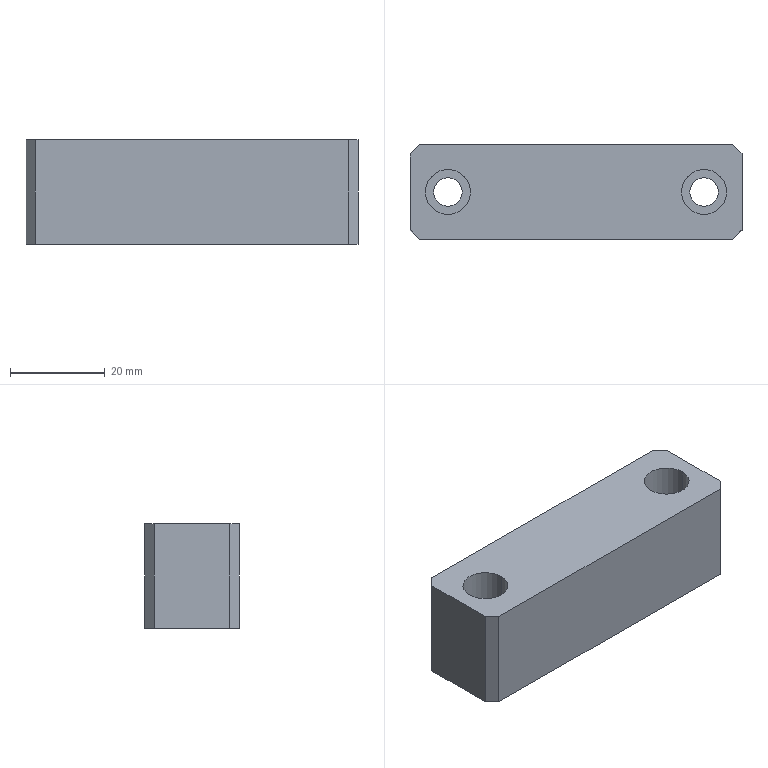Part | SolidWorks | features Chamfer 1, Extrusion 1, HoleWzd 1 | 1 solid | 20 faces | box 70 x 20 x 22 mm | volume 28656 mm3 | plane 12 | cylinder 8 | commonest cylinder face diameters 6 x4 9.5 x4
STEP:
#1=CARTESIAN_POINT('',(-29.44,2.003,1.5));
#2=VERTEX_POINT('',#1);
#3=CARTESIAN_POINT('',(-19.94,2.003,1.5));
#4=VERTEX_POINT('',#3);
#5=CARTESIAN_POINT('',(-24.69,2.003,1.5));
#6=DIRECTION('',(0.,0.,1.));
#7=DIRECTION('',(1.,0.,0.));
#8=AXIS2_PLACEMENT_3D('',#5,#6,#7);
#9=CIRCLE('',#8,4.75);
#10=EDGE_CURVE('',#2,#4,#9,.T.);
#11=ORIENTED_EDGE('',*,*,#10,.F.);
#12=CARTESIAN_POINT('',(-29.44,2.003,10.));
#13=VERTEX_POINT('',#12);
#14=CARTESIAN_POINT('',(-29.44,2.003,10.));
#15=DIRECTION('',(0.,0.,1.));
#16=VECTOR('',#15,1000.);
#17=LINE('',#14,#16);
#18=EDGE_CURVE('',#2,#13,#17,.T.);
#19=ORIENTED_EDGE('',*,*,#18,.T.);
#20=CARTESIAN_POINT('',(-19.94,2.003,10.));
#21=VERTEX_POINT('',#20);
#22=CARTESIAN_POINT('',(-24.69,2.003,10.));
#23=DIRECTION('',(0.,0.,1.));
#24=DIRECTION('',(1.,0.,0.));
#25=AXIS2_PLACEMENT_3D('',#22,#23,#24);
#26=CIRCLE('',#25,4.75);
#27=EDGE_CURVE('',#13,#21,#26,.T.);
#28=ORIENTED_EDGE('',*,*,#27,.T.);
#29=CARTESIAN_POINT('',(-19.94,2.003,10.));
#30=DIRECTION('',(0.,0.,1.));
#31=VECTOR('',#30,1000.);
#32=LINE('',#29,#31);
#33=EDGE_CURVE('',#4,#21,#32,.T.);
#34=ORIENTED_EDGE('',*,*,#33,.F.);
#35=EDGE_LOOP('',(#11,#19,#28,#34));
#36=FACE_OUTER_BOUND('',#35,.T.);
#37=CARTESIAN_POINT('',(-24.69,2.003,10.));
#38=DIRECTION('',(0.,0.,1.));
#39=DIRECTION('',(1.,0.,0.));
#40=AXIS2_PLACEMENT_3D('',#37,#38,#39);
#41=CYLINDRICAL_SURFACE('',#40,4.75);
#42=ADVANCED_FACE('',(#36),#41,.F.);
#43=CARTESIAN_POINT('',(-27.69,2.003,-12.));
#44=VERTEX_POINT('',#43);
#45=CARTESIAN_POINT('',(-21.69,2.003,-12.));
#46=VERTEX_POINT('',#45);
#47=CARTESIAN_POINT('',(-24.69,2.003,-12.));
#48=DIRECTION('',(0.,0.,1.));
#49=DIRECTION('',(1.,0.,0.));
#50=AXIS2_PLACEMENT_3D('',#47,#48,#49);
#51=CIRCLE('',#50,3.);
#52=EDGE_CURVE('',#44,#46,#51,.T.);
#53=ORIENTED_EDGE('',*,*,#52,.F.);
#54=CARTESIAN_POINT('',(-27.69,2.003,1.5));
#55=VERTEX_POINT('',#54);
#56=CARTESIAN_POINT('',(-27.69,2.003,10.));
#57=DIRECTION('',(0.,0.,1.));
#58=VECTOR('',#57,1000.);
#59=LINE('',#56,#58);
#60=EDGE_CURVE('',#44,#55,#59,.T.);
#61=ORIENTED_EDGE('',*,*,#60,.T.);
#62=CARTESIAN_POINT('',(-21.69,2.003,1.5));
#63=VERTEX_POINT('',#62);
#64=CARTESIAN_POINT('',(-24.69,2.003,1.5));
#65=DIRECTION('',(0.,0.,1.));
#66=DIRECTION('',(1.,0.,0.));
#67=AXIS2_PLACEMENT_3D('',#64,#65,#66);
#68=CIRCLE('',#67,3.);
#69=EDGE_CURVE('',#55,#63,#68,.T.);
#70=ORIENTED_EDGE('',*,*,#69,.T.);
#71=CARTESIAN_POINT('',(-21.69,2.003,10.));
#72=DIRECTION('',(0.,0.,1.));
#73=VECTOR('',#72,1000.);
#74=LINE('',#71,#73);
#75=EDGE_CURVE('',#46,#63,#74,.T.);
#76=ORIENTED_EDGE('',*,*,#75,.F.);
#77=EDGE_LOOP('',(#53,#61,#70,#76));
#78=FACE_OUTER_BOUND('',#77,.T.);
#79=CARTESIAN_POINT('',(-24.69,2.003,10.));
#80=DIRECTION('',(0.,0.,1.));
#81=DIRECTION('',(1.,0.,0.));
#82=AXIS2_PLACEMENT_3D('',#79,#80,#81);
#83=CYLINDRICAL_SURFACE('',#82,3.);
#84=ADVANCED_FACE('',(#78),#83,.F.);
#85=CARTESIAN_POINT('',(24.56,2.003,1.5));
#86=VERTEX_POINT('',#85);
#87=CARTESIAN_POINT('',(34.06,2.003,1.5));
#88=VERTEX_POINT('',#87);
#89=CARTESIAN_POINT('',(29.31,2.003,1.5));
#90=DIRECTION('',(0.,0.,1.));
#91=DIRECTION('',(1.,0.,0.));
#92=AXIS2_PLACEMENT_3D('',#89,#90,#91);
#93=CIRCLE('',#92,4.75);
#94=EDGE_CURVE('',#86,#88,#93,.T.);
#95=ORIENTED_EDGE('',*,*,#94,.F.);
#96=CARTESIAN_POINT('',(24.56,2.003,10.));
#97=VERTEX_POINT('',#96);
#98=CARTESIAN_POINT('',(24.56,2.003,10.));
#99=DIRECTION('',(0.,0.,1.));
#100=VECTOR('',#99,1000.);
#101=LINE('',#98,#100);
#102=EDGE_CURVE('',#86,#97,#101,.T.);
#103=ORIENTED_EDGE('',*,*,#102,.T.);
#104=CARTESIAN_POINT('',(34.06,2.003,10.));
#105=VERTEX_POINT('',#104);
#106=CARTESIAN_POINT('',(29.31,2.003,10.));
#107=DIRECTION('',(0.,0.,1.));
#108=DIRECTION('',(1.,0.,0.));
#109=AXIS2_PLACEMENT_3D('',#106,#107,#108);
#110=CIRCLE('',#109,4.75);
#111=EDGE_CURVE('',#97,#105,#110,.T.);
#112=ORIENTED_EDGE('',*,*,#111,.T.);
#113=CARTESIAN_POINT('',(34.06,2.003,10.));
#114=DIRECTION('',(0.,0.,1.));
#115=VECTOR('',#114,1000.);
#116=LINE('',#113,#115);
#117=EDGE_CURVE('',#88,#105,#116,.T.);
#118=ORIENTED_EDGE('',*,*,#117,.F.);
#119=EDGE_LOOP('',(#95,#103,#112,#118));
#120=FACE_OUTER_BOUND('',#119,.T.);
#121=CARTESIAN_POINT('',(29.31,2.003,10.));
#122=DIRECTION('',(0.,0.,1.));
#123=DIRECTION('',(1.,0.,0.));
#124=AXIS2_PLACEMENT_3D('',#121,#122,#123);
#125=CYLINDRICAL_SURFACE('',#124,4.75);
#126=ADVANCED_FACE('',(#120),#125,.F.);
#127=CARTESIAN_POINT('',(26.31,2.003,-12.));
#128=VERTEX_POINT('',#127);
#129=CARTESIAN_POINT('',(32.31,2.003,-12.));
#130=VERTEX_POINT('',#129);
#131=CARTESIAN_POINT('',(29.31,2.003,-12.));
#132=DIRECTION('',(0.,0.,1.));
#133=DIRECTION('',(1.,0.,0.));
#134=AXIS2_PLACEMENT_3D('',#131,#132,#133);
#135=CIRCLE('',#134,3.);
#136=EDGE_CURVE('',#128,#130,#135,.T.);
#137=ORIENTED_EDGE('',*,*,#136,.F.);
#138=CARTESIAN_POINT('',(26.31,2.003,1.5));
#139=VERTEX_POINT('',#138);
#140=CARTESIAN_POINT('',(26.31,2.003,10.));
#141=DIRECTION('',(0.,0.,1.));
#142=VECTOR('',#141,1000.);
#143=LINE('',#140,#142);
#144=EDGE_CURVE('',#128,#139,#143,.T.);
#145=ORIENTED_EDGE('',*,*,#144,.T.);
#146=CARTESIAN_POINT('',(32.31,2.003,1.5));
#147=VERTEX_POINT('',#146);
#148=CARTESIAN_POINT('',(29.31,2.003,1.5));
#149=DIRECTION('',(0.,0.,1.));
#150=DIRECTION('',(1.,0.,0.));
#151=AXIS2_PLACEMENT_3D('',#148,#149,#150);
#152=CIRCLE('',#151,3.);
#153=EDGE_CURVE('',#139,#147,#152,.T.);
#154=ORIENTED_EDGE('',*,*,#153,.T.);
#155=CARTESIAN_POINT('',(32.31,2.003,10.));
#156=DIRECTION('',(0.,0.,1.));
#157=VECTOR('',#156,1000.);
#158=LINE('',#155,#157);
#159=EDGE_CURVE('',#130,#147,#158,.T.);
#160=ORIENTED_EDGE('',*,*,#159,.F.);
#161=EDGE_LOOP('',(#137,#145,#154,#160));
#162=FACE_OUTER_BOUND('',#161,.T.);
#163=CARTESIAN_POINT('',(29.31,2.003,10.));
#164=DIRECTION('',(0.,0.,1.));
#165=DIRECTION('',(1.,0.,0.));
#166=AXIS2_PLACEMENT_3D('',#163,#164,#165);
#167=CYLINDRICAL_SURFACE('',#166,3.);
#168=ADVANCED_FACE('',(#162),#167,.F.);
#169=CARTESIAN_POINT('',(-32.69,10.003,-12.));
#170=VERTEX_POINT('',#169);
#171=CARTESIAN_POINT('',(-32.69,-5.997,-12.));
#172=VERTEX_POINT('',#171);
#173=CARTESIAN_POINT('',(-32.69,12.003,-12.));
#174=DIRECTION('',(0.,-1.,0.));
#175=VECTOR('',#174,1000.);
#176=LINE('',#173,#175);
#177=EDGE_CURVE('',#170,#172,#176,.T.);
#178=ORIENTED_EDGE('',*,*,#177,.T.);
#179=CARTESIAN_POINT('',(-32.69,-5.997,10.));
#180=VERTEX_POINT('',#179);
#181=CARTESIAN_POINT('',(-32.69,-5.997,-12.));
#182=DIRECTION('',(0.,0.,1.));
#183=VECTOR('',#182,1000.);
#184=LINE('',#181,#183);
#185=EDGE_CURVE('',#172,#180,#184,.T.);
#186=ORIENTED_EDGE('',*,*,#185,.T.);
#187=CARTESIAN_POINT('',(-32.69,10.003,10.));
#188=VERTEX_POINT('',#187);
#189=CARTESIAN_POINT('',(-32.69,12.003,10.));
#190=DIRECTION('',(0.,-1.,0.));
#191=VECTOR('',#190,1000.);
#192=LINE('',#189,#191);
#193=EDGE_CURVE('',#188,#180,#192,.T.);
#194=ORIENTED_EDGE('',*,*,#193,.F.);
#195=CARTESIAN_POINT('',(-32.69,10.003,-12.));
#196=DIRECTION('',(0.,0.,-1.));
#197=VECTOR('',#196,1000.);
#198=LINE('',#195,#197);
#199=EDGE_CURVE('',#188,#170,#198,.T.);
#200=ORIENTED_EDGE('',*,*,#199,.T.);
#201=EDGE_LOOP('',(#178,#186,#194,#200));
#202=FACE_OUTER_BOUND('',#201,.T.);
#203=CARTESIAN_POINT('',(-32.69,12.003,-12.));
#204=DIRECTION('',(-1.,0.,0.));
#205=DIRECTION('',(0.,-1.,0.));
#206=AXIS2_PLACEMENT_3D('',#203,#204,#205);
#207=PLANE('',#206);
#208=ADVANCED_FACE('',(#202),#207,.T.);
#209=CARTESIAN_POINT('',(35.31,12.003,10.));
#210=VERTEX_POINT('',#209);
#211=CARTESIAN_POINT('',(-30.69,12.003,10.));
#212=VERTEX_POINT('',#211);
#213=CARTESIAN_POINT('',(-32.69,12.003,10.));
#214=DIRECTION('',(-1.,0.,0.));
#215=VECTOR('',#214,1000.);
#216=LINE('',#213,#215);
#217=EDGE_CURVE('',#210,#212,#216,.T.);
#218=ORIENTED_EDGE('',*,*,#217,.F.);
#219=CARTESIAN_POINT('',(35.31,12.003,-12.));
#220=VERTEX_POINT('',#219);
#221=CARTESIAN_POINT('',(35.31,12.003,-12.));
#222=DIRECTION('',(0.,0.,-1.));
#223=VECTOR('',#222,1000.);
#224=LINE('',#221,#223);
#225=EDGE_CURVE('',#210,#220,#224,.T.);
#226=ORIENTED_EDGE('',*,*,#225,.T.);
#227=CARTESIAN_POINT('',(-30.69,12.003,-12.));
#228=VERTEX_POINT('',#227);
#229=CARTESIAN_POINT('',(-32.69,12.003,-12.));
#230=DIRECTION('',(-1.,0.,0.));
#231=VECTOR('',#230,1000.);
#232=LINE('',#229,#231);
#233=EDGE_CURVE('',#220,#228,#232,.T.);
#234=ORIENTED_EDGE('',*,*,#233,.T.);
#235=CARTESIAN_POINT('',(-30.69,12.003,-12.));
#236=DIRECTION('',(0.,0.,1.));
#237=VECTOR('',#236,1000.);
#238=LINE('',#235,#237);
#239=EDGE_CURVE('',#228,#212,#238,.T.);
#240=ORIENTED_EDGE('',*,*,#239,.T.);
#241=EDGE_LOOP('',(#218,#226,#234,#240));
#242=FACE_OUTER_BOUND('',#241,.T.);
#243=CARTESIAN_POINT('',(-32.69,12.003,-12.));
#244=DIRECTION('',(0.,1.,0.));
#245=DIRECTION('',(0.,0.,1.));
#246=AXIS2_PLACEMENT_3D('',#243,#244,#245);
#247=PLANE('',#246);
#248=ADVANCED_FACE('',(#242),#247,.T.);
#249=CARTESIAN_POINT('',(37.31,-5.997,10.));
#250=VERTEX_POINT('',#249);
#251=CARTESIAN_POINT('',(37.31,10.003,10.));
#252=VERTEX_POINT('',#251);
#253=CARTESIAN_POINT('',(37.31,12.003,10.));
#254=DIRECTION('',(0.,1.,0.));
#255=VECTOR('',#254,1000.);
#256=LINE('',#253,#255);
#257=EDGE_CURVE('',#250,#252,#256,.T.);
#258=ORIENTED_EDGE('',*,*,#257,.F.);
#259=CARTESIAN_POINT('',(37.31,-5.997,-12.));
#260=VERTEX_POINT('',#259);
#261=CARTESIAN_POINT('',(37.31,-5.997,-12.));
#262=DIRECTION('',(0.,0.,-1.));
#263=VECTOR('',#262,1000.);
#264=LINE('',#261,#263);
#265=EDGE_CURVE('',#250,#260,#264,.T.);
#266=ORIENTED_EDGE('',*,*,#265,.T.);
#267=CARTESIAN_POINT('',(37.31,10.003,-12.));
#268=VERTEX_POINT('',#267);
#269=CARTESIAN_POINT('',(37.31,12.003,-12.));
#270=DIRECTION('',(0.,1.,0.));
#271=VECTOR('',#270,1000.);
#272=LINE('',#269,#271);
#273=EDGE_CURVE('',#260,#268,#272,.T.);
#274=ORIENTED_EDGE('',*,*,#273,.T.);
#275=CARTESIAN_POINT('',(37.31,10.003,-12.));
#276=DIRECTION('',(0.,0.,1.));
#277=VECTOR('',#276,1000.);
#278=LINE('',#275,#277);
#279=EDGE_CURVE('',#268,#252,#278,.T.);
#280=ORIENTED_EDGE('',*,*,#279,.T.);
#281=EDGE_LOOP('',(#258,#266,#274,#280));
#282=FACE_OUTER_BOUND('',#281,.T.);
#283=CARTESIAN_POINT('',(37.31,12.003,-12.));
#284=DIRECTION('',(1.,0.,0.));
#285=DIRECTION('',(0.,0.,-1.));
#286=AXIS2_PLACEMENT_3D('',#283,#284,#285);
#287=PLANE('',#286);
#288=ADVANCED_FACE('',(#282),#287,.T.);
#289=CARTESIAN_POINT('',(-30.69,-7.997,-12.));
#290=VERTEX_POINT('',#289);
#291=CARTESIAN_POINT('',(35.31,-7.997,-12.));
#292=VERTEX_POINT('',#291);
#293=CARTESIAN_POINT('',(-32.69,-7.997,-12.));
#294=DIRECTION('',(1.,0.,0.));
#295=VECTOR('',#294,1000.);
#296=LINE('',#293,#295);
#297=EDGE_CURVE('',#290,#292,#296,.T.);
#298=ORIENTED_EDGE('',*,*,#297,.T.);
#299=CARTESIAN_POINT('',(35.31,-7.997,10.));
#300=VERTEX_POINT('',#299);
#301=CARTESIAN_POINT('',(35.31,-7.997,-12.));
#302=DIRECTION('',(0.,0.,1.));
#303=VECTOR('',#302,1000.);
#304=LINE('',#301,#303);
#305=EDGE_CURVE('',#292,#300,#304,.T.);
#306=ORIENTED_EDGE('',*,*,#305,.T.);
#307=CARTESIAN_POINT('',(-30.69,-7.997,10.));
#308=VERTEX_POINT('',#307);
#309=CARTESIAN_POINT('',(-32.69,-7.997,10.));
#310=DIRECTION('',(1.,0.,0.));
#311=VECTOR('',#310,1000.);
#312=LINE('',#309,#311);
#313=EDGE_CURVE('',#308,#300,#312,.T.);
#314=ORIENTED_EDGE('',*,*,#313,.F.);
#315=CARTESIAN_POINT('',(-30.69,-7.997,-12.));
#316=DIRECTION('',(0.,0.,-1.));
#317=VECTOR('',#316,1000.);
#318=LINE('',#315,#317);
#319=EDGE_CURVE('',#308,#290,#318,.T.);
#320=ORIENTED_EDGE('',*,*,#319,.T.);
#321=EDGE_LOOP('',(#298,#306,#314,#320));
#322=FACE_OUTER_BOUND('',#321,.T.);
#323=CARTESIAN_POINT('',(-32.69,-7.997,-12.));
#324=DIRECTION('',(0.,-1.,0.));
#325=DIRECTION('',(0.,0.,-1.));
#326=AXIS2_PLACEMENT_3D('',#323,#324,#325);
#327=PLANE('',#326);
#328=ADVANCED_FACE('',(#322),#327,.T.);
#329=CARTESIAN_POINT('',(-24.69,2.003,-12.));
#330=DIRECTION('',(0.,0.,1.));
#331=DIRECTION('',(1.,0.,0.));
#332=AXIS2_PLACEMENT_3D('',#329,#330,#331);
#333=CIRCLE('',#332,3.);
#334=EDGE_CURVE('',#46,#44,#333,.T.);
#335=ORIENTED_EDGE('',*,*,#334,.T.);
#336=ORIENTED_EDGE('',*,*,#52,.T.);
#337=EDGE_LOOP('',(#335,#336));
#338=FACE_BOUND('',#337,.T.);
#339=CARTESIAN_POINT('',(29.31,2.003,-12.));
#340=DIRECTION('',(0.,0.,1.));
#341=DIRECTION('',(1.,0.,0.));
#342=AXIS2_PLACEMENT_3D('',#339,#340,#341);
#343=CIRCLE('',#342,3.);
#344=EDGE_CURVE('',#130,#128,#343,.T.);
#345=ORIENTED_EDGE('',*,*,#344,.T.);
#346=ORIENTED_EDGE('',*,*,#136,.T.);
#347=EDGE_LOOP('',(#345,#346));
#348=FACE_BOUND('',#347,.T.);
#349=ORIENTED_EDGE('',*,*,#273,.F.);
#350=CARTESIAN_POINT('',(35.31,-7.997,-12.));
#351=DIRECTION('',(-0.7071,-0.7071,0.));
#352=VECTOR('',#351,1000.);
#353=LINE('',#350,#352);
#354=EDGE_CURVE('',#260,#292,#353,.T.);
#355=ORIENTED_EDGE('',*,*,#354,.T.);
#356=ORIENTED_EDGE('',*,*,#297,.F.);
#357=CARTESIAN_POINT('',(-32.69,-5.997,-12.));
#358=DIRECTION('',(-0.7071,0.7071,0.));
#359=VECTOR('',#358,1000.);
#360=LINE('',#357,#359);
#361=EDGE_CURVE('',#290,#172,#360,.T.);
#362=ORIENTED_EDGE('',*,*,#361,.T.);
#363=ORIENTED_EDGE('',*,*,#177,.F.);
#364=CARTESIAN_POINT('',(-30.69,12.003,-12.));
#365=DIRECTION('',(0.7071,0.7071,0.));
#366=VECTOR('',#365,1000.);
#367=LINE('',#364,#366);
#368=EDGE_CURVE('',#170,#228,#367,.T.);
#369=ORIENTED_EDGE('',*,*,#368,.T.);
#370=ORIENTED_EDGE('',*,*,#233,.F.);
#371=CARTESIAN_POINT('',(37.31,10.003,-12.));
#372=DIRECTION('',(0.7071,-0.7071,0.));
#373=VECTOR('',#372,1000.);
#374=LINE('',#371,#373);
#375=EDGE_CURVE('',#220,#268,#374,.T.);
#376=ORIENTED_EDGE('',*,*,#375,.T.);
#377=EDGE_LOOP('',(#349,#355,#356,#362,#363,#369,#370,#376));
#378=FACE_OUTER_BOUND('',#377,.T.);
#379=CARTESIAN_POINT('',(0.,0.,-12.));
#380=DIRECTION('',(0.,0.,1.));
#381=DIRECTION('',(1.,0.,0.));
#382=AXIS2_PLACEMENT_3D('',#379,#380,#381);
#383=PLANE('',#382);
#384=ADVANCED_FACE('',(#338,#348,#378),#383,.F.);
#385=CARTESIAN_POINT('',(-24.69,2.003,10.));
#386=DIRECTION('',(0.,0.,1.));
#387=DIRECTION('',(1.,0.,0.));
#388=AXIS2_PLACEMENT_3D('',#385,#386,#387);
#389=CIRCLE('',#388,4.75);
#390=EDGE_CURVE('',#21,#13,#389,.T.);
#391=ORIENTED_EDGE('',*,*,#390,.F.);
#392=ORIENTED_EDGE('',*,*,#27,.F.);
#393=EDGE_LOOP('',(#391,#392));
#394=FACE_BOUND('',#393,.T.);
#395=CARTESIAN_POINT('',(29.31,2.003,10.));
#396=DIRECTION('',(0.,0.,1.));
#397=DIRECTION('',(1.,0.,0.));
#398=AXIS2_PLACEMENT_3D('',#395,#396,#397);
#399=CIRCLE('',#398,4.75);
#400=EDGE_CURVE('',#105,#97,#399,.T.);
#401=ORIENTED_EDGE('',*,*,#400,.F.);
#402=ORIENTED_EDGE('',*,*,#111,.F.);
#403=EDGE_LOOP('',(#401,#402));
#404=FACE_BOUND('',#403,.T.);
#405=ORIENTED_EDGE('',*,*,#313,.T.);
#406=CARTESIAN_POINT('',(21.653,-21.653,10.));
#407=DIRECTION('',(0.7071,0.7071,0.));
#408=VECTOR('',#407,1000.);
#409=LINE('',#406,#408);
#410=EDGE_CURVE('',#300,#250,#409,.T.);
#411=ORIENTED_EDGE('',*,*,#410,.T.);
#412=ORIENTED_EDGE('',*,*,#257,.T.);
#413=CARTESIAN_POINT('',(23.656,23.656,10.));
#414=DIRECTION('',(-0.7071,0.7071,0.));
#415=VECTOR('',#414,1000.);
#416=LINE('',#413,#415);
#417=EDGE_CURVE('',#252,#210,#416,.T.);
#418=ORIENTED_EDGE('',*,*,#417,.T.);
#419=ORIENTED_EDGE('',*,*,#217,.T.);
#420=CARTESIAN_POINT('',(-21.347,21.347,10.));
#421=DIRECTION('',(-0.7071,-0.7071,0.));
#422=VECTOR('',#421,1000.);
#423=LINE('',#420,#422);
#424=EDGE_CURVE('',#212,#188,#423,.T.);
#425=ORIENTED_EDGE('',*,*,#424,.T.);
#426=ORIENTED_EDGE('',*,*,#193,.T.);
#427=CARTESIAN_POINT('',(-19.344,-19.344,10.));
#428=DIRECTION('',(0.7071,-0.7071,0.));
#429=VECTOR('',#428,1000.);
#430=LINE('',#427,#429);
#431=EDGE_CURVE('',#180,#308,#430,.T.);
#432=ORIENTED_EDGE('',*,*,#431,.T.);
#433=EDGE_LOOP('',(#405,#411,#412,#418,#419,#425,#426,#432));
#434=FACE_OUTER_BOUND('',#433,.T.);
#435=CARTESIAN_POINT('',(0.,0.,10.));
#436=DIRECTION('',(0.,0.,1.));
#437=DIRECTION('',(1.,0.,0.));
#438=AXIS2_PLACEMENT_3D('',#435,#436,#437);
#439=PLANE('',#438);
#440=ADVANCED_FACE('',(#394,#404,#434),#439,.T.);
#441=ORIENTED_EDGE('',*,*,#144,.F.);
#442=ORIENTED_EDGE('',*,*,#344,.F.);
#443=ORIENTED_EDGE('',*,*,#159,.T.);
#444=CARTESIAN_POINT('',(29.31,2.003,1.5));
#445=DIRECTION('',(0.,0.,1.));
#446=DIRECTION('',(1.,0.,0.));
#447=AXIS2_PLACEMENT_3D('',#444,#445,#446);
#448=CIRCLE('',#447,3.);
#449=EDGE_CURVE('',#147,#139,#448,.T.);
#450=ORIENTED_EDGE('',*,*,#449,.T.);
#451=EDGE_LOOP('',(#441,#442,#443,#450));
#452=FACE_OUTER_BOUND('',#451,.T.);
#453=CARTESIAN_POINT('',(29.31,2.003,10.));
#454=DIRECTION('',(0.,0.,1.));
#455=DIRECTION('',(1.,0.,0.));
#456=AXIS2_PLACEMENT_3D('',#453,#454,#455);
#457=CYLINDRICAL_SURFACE('',#456,3.);
#458=ADVANCED_FACE('',(#452),#457,.F.);
#459=ORIENTED_EDGE('',*,*,#449,.F.);
#460=ORIENTED_EDGE('',*,*,#153,.F.);
#461=EDGE_LOOP('',(#459,#460));
#462=FACE_BOUND('',#461,.T.);
#463=CARTESIAN_POINT('',(29.31,2.003,1.5));
#464=DIRECTION('',(0.,0.,1.));
#465=DIRECTION('',(1.,0.,0.));
#466=AXIS2_PLACEMENT_3D('',#463,#464,#465);
#467=CIRCLE('',#466,4.75);
#468=EDGE_CURVE('',#88,#86,#467,.T.);
#469=ORIENTED_EDGE('',*,*,#468,.T.);
#470=ORIENTED_EDGE('',*,*,#94,.T.);
#471=EDGE_LOOP('',(#469,#470));
#472=FACE_OUTER_BOUND('',#471,.T.);
#473=CARTESIAN_POINT('',(32.31,2.003,1.5));
#474=DIRECTION('',(0.,0.,-1.));
#475=DIRECTION('',(-1.,0.,0.));
#476=AXIS2_PLACEMENT_3D('',#473,#474,#475);
#477=PLANE('',#476);
#478=ADVANCED_FACE('',(#462,#472),#477,.F.);
#479=ORIENTED_EDGE('',*,*,#102,.F.);
#480=ORIENTED_EDGE('',*,*,#468,.F.);
#481=ORIENTED_EDGE('',*,*,#117,.T.);
#482=ORIENTED_EDGE('',*,*,#400,.T.);
#483=EDGE_LOOP('',(#479,#480,#481,#482));
#484=FACE_OUTER_BOUND('',#483,.T.);
#485=CARTESIAN_POINT('',(29.31,2.003,10.));
#486=DIRECTION('',(0.,0.,1.));
#487=DIRECTION('',(1.,0.,0.));
#488=AXIS2_PLACEMENT_3D('',#485,#486,#487);
#489=CYLINDRICAL_SURFACE('',#488,4.75);
#490=ADVANCED_FACE('',(#484),#489,.F.);
#491=ORIENTED_EDGE('',*,*,#60,.F.);
#492=ORIENTED_EDGE('',*,*,#334,.F.);
#493=ORIENTED_EDGE('',*,*,#75,.T.);
#494=CARTESIAN_POINT('',(-24.69,2.003,1.5));
#495=DIRECTION('',(0.,0.,1.));
#496=DIRECTION('',(1.,0.,0.));
#497=AXIS2_PLACEMENT_3D('',#494,#495,#496);
#498=CIRCLE('',#497,3.);
#499=EDGE_CURVE('',#63,#55,#498,.T.);
#500=ORIENTED_EDGE('',*,*,#499,.T.);
#501=EDGE_LOOP('',(#491,#492,#493,#500));
#502=FACE_OUTER_BOUND('',#501,.T.);
#503=CARTESIAN_POINT('',(-24.69,2.003,10.));
#504=DIRECTION('',(0.,0.,1.));
#505=DIRECTION('',(1.,0.,0.));
#506=AXIS2_PLACEMENT_3D('',#503,#504,#505);
#507=CYLINDRICAL_SURFACE('',#506,3.);
#508=ADVANCED_FACE('',(#502),#507,.F.);
#509=ORIENTED_EDGE('',*,*,#499,.F.);
#510=ORIENTED_EDGE('',*,*,#69,.F.);
#511=EDGE_LOOP('',(#509,#510));
#512=FACE_BOUND('',#511,.T.);
#513=CARTESIAN_POINT('',(-24.69,2.003,1.5));
#514=DIRECTION('',(0.,0.,1.));
#515=DIRECTION('',(1.,0.,0.));
#516=AXIS2_PLACEMENT_3D('',#513,#514,#515);
#517=CIRCLE('',#516,4.75);
#518=EDGE_CURVE('',#4,#2,#517,.T.);
#519=ORIENTED_EDGE('',*,*,#518,.T.);
#520=ORIENTED_EDGE('',*,*,#10,.T.);
#521=EDGE_LOOP('',(#519,#520));
#522=FACE_OUTER_BOUND('',#521,.T.);
#523=CARTESIAN_POINT('',(-21.69,2.003,1.5));
#524=DIRECTION('',(0.,0.,-1.));
#525=DIRECTION('',(-1.,0.,0.));
#526=AXIS2_PLACEMENT_3D('',#523,#524,#525);
#527=PLANE('',#526);
#528=ADVANCED_FACE('',(#512,#522),#527,.F.);
#529=ORIENTED_EDGE('',*,*,#18,.F.);
#530=ORIENTED_EDGE('',*,*,#518,.F.);
#531=ORIENTED_EDGE('',*,*,#33,.T.);
#532=ORIENTED_EDGE('',*,*,#390,.T.);
#533=EDGE_LOOP('',(#529,#530,#531,#532));
#534=FACE_OUTER_BOUND('',#533,.T.);
#535=CARTESIAN_POINT('',(-24.69,2.003,10.));
#536=DIRECTION('',(0.,0.,1.));
#537=DIRECTION('',(1.,0.,0.));
#538=AXIS2_PLACEMENT_3D('',#535,#536,#537);
#539=CYLINDRICAL_SURFACE('',#538,4.75);
#540=ADVANCED_FACE('',(#534),#539,.F.);
#541=ORIENTED_EDGE('',*,*,#354,.F.);
#542=ORIENTED_EDGE('',*,*,#265,.F.);
#543=ORIENTED_EDGE('',*,*,#410,.F.);
#544=ORIENTED_EDGE('',*,*,#305,.F.);
#545=EDGE_LOOP('',(#541,#542,#543,#544));
#546=FACE_OUTER_BOUND('',#545,.T.);
#547=CARTESIAN_POINT('',(35.31,-7.997,-12.));
#548=DIRECTION('',(-0.7071,0.7071,0.));
#549=DIRECTION('',(0.,0.,1.));
#550=AXIS2_PLACEMENT_3D('',#547,#548,#549);
#551=PLANE('',#550);
#552=ADVANCED_FACE('',(#546),#551,.F.);
#553=ORIENTED_EDGE('',*,*,#375,.F.);
#554=ORIENTED_EDGE('',*,*,#225,.F.);
#555=ORIENTED_EDGE('',*,*,#417,.F.);
#556=ORIENTED_EDGE('',*,*,#279,.F.);
#557=EDGE_LOOP('',(#553,#554,#555,#556));
#558=FACE_OUTER_BOUND('',#557,.T.);
#559=CARTESIAN_POINT('',(37.31,10.003,-12.));
#560=DIRECTION('',(-0.7071,-0.7071,0.));
#561=DIRECTION('',(0.,0.,1.));
#562=AXIS2_PLACEMENT_3D('',#559,#560,#561);
#563=PLANE('',#562);
#564=ADVANCED_FACE('',(#558),#563,.F.);
#565=ORIENTED_EDGE('',*,*,#361,.F.);
#566=ORIENTED_EDGE('',*,*,#319,.F.);
#567=ORIENTED_EDGE('',*,*,#431,.F.);
#568=ORIENTED_EDGE('',*,*,#185,.F.);
#569=EDGE_LOOP('',(#565,#566,#567,#568));
#570=FACE_OUTER_BOUND('',#569,.T.);
#571=CARTESIAN_POINT('',(-32.69,-5.997,-12.));
#572=DIRECTION('',(0.7071,0.7071,0.));
#573=DIRECTION('',(0.,0.,1.));
#574=AXIS2_PLACEMENT_3D('',#571,#572,#573);
#575=PLANE('',#574);
#576=ADVANCED_FACE('',(#570),#575,.F.);
#577=ORIENTED_EDGE('',*,*,#368,.F.);
#578=ORIENTED_EDGE('',*,*,#199,.F.);
#579=ORIENTED_EDGE('',*,*,#424,.F.);
#580=ORIENTED_EDGE('',*,*,#239,.F.);
#581=EDGE_LOOP('',(#577,#578,#579,#580));
#582=FACE_OUTER_BOUND('',#581,.T.);
#583=CARTESIAN_POINT('',(-30.69,12.003,-12.));
#584=DIRECTION('',(0.7071,-0.7071,0.));
#585=DIRECTION('',(0.,0.,1.));
#586=AXIS2_PLACEMENT_3D('',#583,#584,#585);
#587=PLANE('',#586);
#588=ADVANCED_FACE('',(#582),#587,.F.);
#589=CLOSED_SHELL('',(#42,#84,#126,#168,#208,#248,#288,#328,#384,#440,#458,#478,#490,#508,#528,#540,#552,#564,#576,#588));
#590=MANIFOLD_SOLID_BREP('',#589);
#591=CARTESIAN_POINT('',(0.,0.,0.));
#592=DIRECTION('',(0.,0.,1.));
#593=DIRECTION('',(1.,0.,0.));
#594=AXIS2_PLACEMENT_3D('',#591,#592,#593);
#595=(LENGTH_UNIT()NAMED_UNIT(*)SI_UNIT(.MILLI.,.METRE.));
#596=UNCERTAINTY_MEASURE_WITH_UNIT(LENGTH_MEASURE(0.00001),#595,'','');
#597=(NAMED_UNIT(*)PLANE_ANGLE_UNIT()SI_UNIT($,.RADIAN.));
#598=(NAMED_UNIT(*)SI_UNIT($,.STERADIAN.)SOLID_ANGLE_UNIT());
#599=(GEOMETRIC_REPRESENTATION_CONTEXT(3)GLOBAL_UNCERTAINTY_ASSIGNED_CONTEXT((#596))GLOBAL_UNIT_ASSIGNED_CONTEXT((#595,#597,#598))REPRESENTATION_CONTEXT('',''));
#600=ADVANCED_BREP_SHAPE_REPRESENTATION('',(#590,#594),#599);